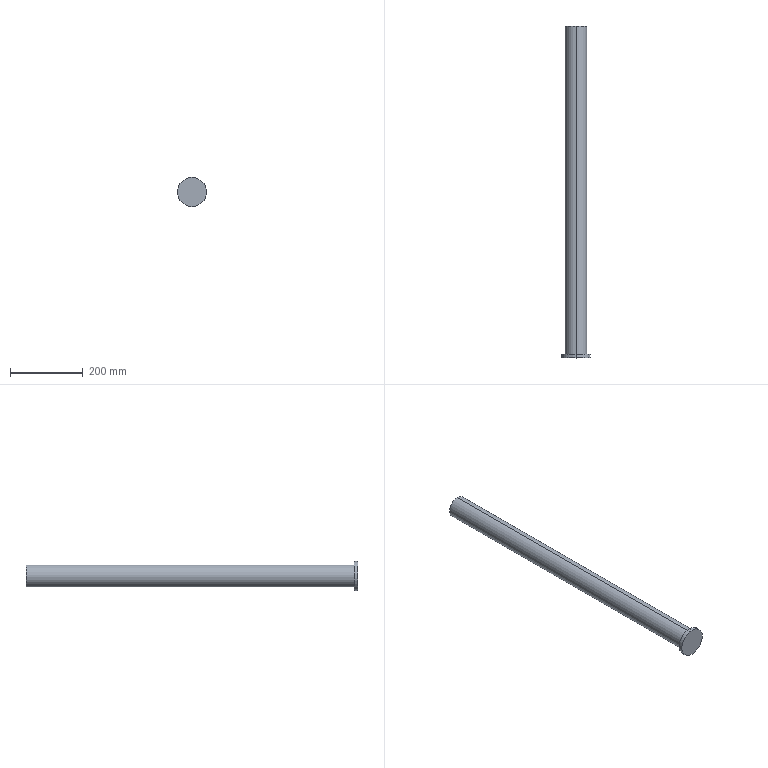Part | STEP file | Tie rod | 1 solid | 10 faces | box 80 x 910 x 80 mm | volume 827810 mm3 | cylinder 6 | plane 4 | commonest cylinder face diameters 50 x2 60 x2 80 x2
STEP:
#1=CARTESIAN_POINT('',(0.,910.,-25.));
#2=VERTEX_POINT('',#1);
#3=CARTESIAN_POINT('',(0.,910.,25.));
#4=VERTEX_POINT('',#3);
#5=CARTESIAN_POINT('',(0.,910.,0.));
#6=DIRECTION('',(0.,1.,0.));
#7=DIRECTION('',(0.,0.,1.));
#8=AXIS2_PLACEMENT_3D('',#5,#6,#7);
#9=CIRCLE('',#8,25.);
#10=EDGE_CURVE('',#2,#4,#9,.T.);
#11=ORIENTED_EDGE('',*,*,#10,.T.);
#12=CARTESIAN_POINT('',(0.,10.,25.));
#13=VERTEX_POINT('',#12);
#14=CARTESIAN_POINT('',(0.,910.,25.));
#15=DIRECTION('',(0.,-1.,0.));
#16=VECTOR('',#15,1000.);
#17=LINE('',#14,#16);
#18=EDGE_CURVE('',#4,#13,#17,.T.);
#19=ORIENTED_EDGE('',*,*,#18,.T.);
#20=CARTESIAN_POINT('',(0.,10.,-25.));
#21=VERTEX_POINT('',#20);
#22=CARTESIAN_POINT('',(0.,10.,0.));
#23=DIRECTION('',(0.,-1.,0.));
#24=DIRECTION('',(0.,0.,1.));
#25=AXIS2_PLACEMENT_3D('',#22,#23,#24);
#26=CIRCLE('',#25,25.);
#27=EDGE_CURVE('',#13,#21,#26,.T.);
#28=ORIENTED_EDGE('',*,*,#27,.T.);
#29=CARTESIAN_POINT('',(0.,910.,-25.));
#30=DIRECTION('',(0.,-1.,0.));
#31=VECTOR('',#30,1000.);
#32=LINE('',#29,#31);
#33=EDGE_CURVE('',#2,#21,#32,.T.);
#34=ORIENTED_EDGE('',*,*,#33,.F.);
#35=EDGE_LOOP('',(#11,#19,#28,#34));
#36=FACE_OUTER_BOUND('',#35,.T.);
#37=CARTESIAN_POINT('',(0.,910.,0.));
#38=DIRECTION('',(0.,-1.,0.));
#39=DIRECTION('',(0.,0.,-1.));
#40=AXIS2_PLACEMENT_3D('',#37,#38,#39);
#41=CYLINDRICAL_SURFACE('',#40,25.);
#42=ADVANCED_FACE('',(#36),#41,.F.);
#43=CARTESIAN_POINT('',(0.,910.,30.));
#44=VERTEX_POINT('',#43);
#45=CARTESIAN_POINT('',(0.,910.,-30.));
#46=VERTEX_POINT('',#45);
#47=CARTESIAN_POINT('',(0.,910.,0.));
#48=DIRECTION('',(0.,1.,0.));
#49=DIRECTION('',(0.,0.,1.));
#50=AXIS2_PLACEMENT_3D('',#47,#48,#49);
#51=CIRCLE('',#50,30.);
#52=EDGE_CURVE('',#44,#46,#51,.T.);
#53=ORIENTED_EDGE('',*,*,#52,.F.);
#54=CARTESIAN_POINT('',(0.,10.,30.));
#55=VERTEX_POINT('',#54);
#56=CARTESIAN_POINT('',(0.,910.,30.));
#57=DIRECTION('',(0.,-1.,0.));
#58=VECTOR('',#57,1000.);
#59=LINE('',#56,#58);
#60=EDGE_CURVE('',#44,#55,#59,.T.);
#61=ORIENTED_EDGE('',*,*,#60,.T.);
#62=CARTESIAN_POINT('',(0.,10.,-30.));
#63=VERTEX_POINT('',#62);
#64=CARTESIAN_POINT('',(0.,10.,0.));
#65=DIRECTION('',(0.,1.,0.));
#66=DIRECTION('',(0.,0.,1.));
#67=AXIS2_PLACEMENT_3D('',#64,#65,#66);
#68=CIRCLE('',#67,30.);
#69=EDGE_CURVE('',#55,#63,#68,.T.);
#70=ORIENTED_EDGE('',*,*,#69,.T.);
#71=CARTESIAN_POINT('',(0.,910.,-30.));
#72=DIRECTION('',(0.,-1.,0.));
#73=VECTOR('',#72,1000.);
#74=LINE('',#71,#73);
#75=EDGE_CURVE('',#46,#63,#74,.T.);
#76=ORIENTED_EDGE('',*,*,#75,.F.);
#77=EDGE_LOOP('',(#53,#61,#70,#76));
#78=FACE_OUTER_BOUND('',#77,.T.);
#79=CARTESIAN_POINT('',(0.,910.,0.));
#80=DIRECTION('',(0.,-1.,0.));
#81=DIRECTION('',(0.,0.,-1.));
#82=AXIS2_PLACEMENT_3D('',#79,#80,#81);
#83=CYLINDRICAL_SURFACE('',#82,30.);
#84=ADVANCED_FACE('',(#78),#83,.T.);
#85=CARTESIAN_POINT('',(0.,10.,40.));
#86=VERTEX_POINT('',#85);
#87=CARTESIAN_POINT('',(0.,10.,-40.));
#88=VERTEX_POINT('',#87);
#89=CARTESIAN_POINT('',(0.,10.,0.));
#90=DIRECTION('',(0.,1.,0.));
#91=DIRECTION('',(0.,0.,1.));
#92=AXIS2_PLACEMENT_3D('',#89,#90,#91);
#93=CIRCLE('',#92,40.);
#94=EDGE_CURVE('',#86,#88,#93,.T.);
#95=ORIENTED_EDGE('',*,*,#94,.F.);
#96=CARTESIAN_POINT('',(0.,0.,40.));
#97=VERTEX_POINT('',#96);
#98=CARTESIAN_POINT('',(0.,10.,40.));
#99=DIRECTION('',(0.,-1.,0.));
#100=VECTOR('',#99,1000.);
#101=LINE('',#98,#100);
#102=EDGE_CURVE('',#86,#97,#101,.T.);
#103=ORIENTED_EDGE('',*,*,#102,.T.);
#104=CARTESIAN_POINT('',(0.,0.,-40.));
#105=VERTEX_POINT('',#104);
#106=CARTESIAN_POINT('',(0.,0.,0.));
#107=DIRECTION('',(0.,1.,0.));
#108=DIRECTION('',(0.,0.,1.));
#109=AXIS2_PLACEMENT_3D('',#106,#107,#108);
#110=CIRCLE('',#109,40.);
#111=EDGE_CURVE('',#97,#105,#110,.T.);
#112=ORIENTED_EDGE('',*,*,#111,.T.);
#113=CARTESIAN_POINT('',(0.,10.,-40.));
#114=DIRECTION('',(0.,-1.,0.));
#115=VECTOR('',#114,1000.);
#116=LINE('',#113,#115);
#117=EDGE_CURVE('',#88,#105,#116,.T.);
#118=ORIENTED_EDGE('',*,*,#117,.F.);
#119=EDGE_LOOP('',(#95,#103,#112,#118));
#120=FACE_OUTER_BOUND('',#119,.T.);
#121=CARTESIAN_POINT('',(0.,10.,0.));
#122=DIRECTION('',(0.,-1.,0.));
#123=DIRECTION('',(0.,0.,-1.));
#124=AXIS2_PLACEMENT_3D('',#121,#122,#123);
#125=CYLINDRICAL_SURFACE('',#124,40.);
#126=ADVANCED_FACE('',(#120),#125,.T.);
#127=ORIENTED_EDGE('',*,*,#102,.F.);
#128=CARTESIAN_POINT('',(0.,10.,0.));
#129=DIRECTION('',(0.,1.,0.));
#130=DIRECTION('',(0.,0.,1.));
#131=AXIS2_PLACEMENT_3D('',#128,#129,#130);
#132=CIRCLE('',#131,40.);
#133=EDGE_CURVE('',#88,#86,#132,.T.);
#134=ORIENTED_EDGE('',*,*,#133,.F.);
#135=ORIENTED_EDGE('',*,*,#117,.T.);
#136=CARTESIAN_POINT('',(0.,0.,0.));
#137=DIRECTION('',(0.,1.,0.));
#138=DIRECTION('',(0.,0.,1.));
#139=AXIS2_PLACEMENT_3D('',#136,#137,#138);
#140=CIRCLE('',#139,40.);
#141=EDGE_CURVE('',#105,#97,#140,.T.);
#142=ORIENTED_EDGE('',*,*,#141,.T.);
#143=EDGE_LOOP('',(#127,#134,#135,#142));
#144=FACE_OUTER_BOUND('',#143,.T.);
#145=CARTESIAN_POINT('',(0.,10.,0.));
#146=DIRECTION('',(0.,-1.,0.));
#147=DIRECTION('',(0.,0.,-1.));
#148=AXIS2_PLACEMENT_3D('',#145,#146,#147);
#149=CYLINDRICAL_SURFACE('',#148,40.);
#150=ADVANCED_FACE('',(#144),#149,.T.);
#151=CARTESIAN_POINT('',(0.,10.,0.));
#152=DIRECTION('',(0.,1.,0.));
#153=DIRECTION('',(0.,0.,1.));
#154=AXIS2_PLACEMENT_3D('',#151,#152,#153);
#155=CIRCLE('',#154,30.);
#156=EDGE_CURVE('',#63,#55,#155,.T.);
#157=ORIENTED_EDGE('',*,*,#156,.F.);
#158=ORIENTED_EDGE('',*,*,#69,.F.);
#159=EDGE_LOOP('',(#157,#158));
#160=FACE_BOUND('',#159,.T.);
#161=ORIENTED_EDGE('',*,*,#133,.T.);
#162=ORIENTED_EDGE('',*,*,#94,.T.);
#163=EDGE_LOOP('',(#161,#162));
#164=FACE_OUTER_BOUND('',#163,.T.);
#165=CARTESIAN_POINT('',(0.,10.,0.));
#166=DIRECTION('',(0.,1.,0.));
#167=DIRECTION('',(0.,0.,1.));
#168=AXIS2_PLACEMENT_3D('',#165,#166,#167);
#169=PLANE('',#168);
#170=ADVANCED_FACE('',(#160,#164),#169,.T.);
#171=ORIENTED_EDGE('',*,*,#141,.F.);
#172=ORIENTED_EDGE('',*,*,#111,.F.);
#173=EDGE_LOOP('',(#171,#172));
#174=FACE_OUTER_BOUND('',#173,.T.);
#175=CARTESIAN_POINT('',(0.,0.,0.));
#176=DIRECTION('',(0.,1.,0.));
#177=DIRECTION('',(0.,0.,1.));
#178=AXIS2_PLACEMENT_3D('',#175,#176,#177);
#179=PLANE('',#178);
#180=ADVANCED_FACE('',(#174),#179,.F.);
#181=CARTESIAN_POINT('',(0.,910.,0.));
#182=DIRECTION('',(0.,1.,0.));
#183=DIRECTION('',(0.,0.,1.));
#184=AXIS2_PLACEMENT_3D('',#181,#182,#183);
#185=CIRCLE('',#184,30.);
#186=EDGE_CURVE('',#46,#44,#185,.T.);
#187=ORIENTED_EDGE('',*,*,#186,.T.);
#188=ORIENTED_EDGE('',*,*,#52,.T.);
#189=EDGE_LOOP('',(#187,#188));
#190=FACE_OUTER_BOUND('',#189,.T.);
#191=ORIENTED_EDGE('',*,*,#10,.F.);
#192=CARTESIAN_POINT('',(0.,910.,0.));
#193=DIRECTION('',(0.,1.,0.));
#194=DIRECTION('',(0.,0.,1.));
#195=AXIS2_PLACEMENT_3D('',#192,#193,#194);
#196=CIRCLE('',#195,25.);
#197=EDGE_CURVE('',#4,#2,#196,.T.);
#198=ORIENTED_EDGE('',*,*,#197,.F.);
#199=EDGE_LOOP('',(#191,#198));
#200=FACE_BOUND('',#199,.T.);
#201=CARTESIAN_POINT('',(0.,910.,0.));
#202=DIRECTION('',(0.,1.,0.));
#203=DIRECTION('',(0.,0.,1.));
#204=AXIS2_PLACEMENT_3D('',#201,#202,#203);
#205=PLANE('',#204);
#206=ADVANCED_FACE('',(#190,#200),#205,.T.);
#207=ORIENTED_EDGE('',*,*,#60,.F.);
#208=ORIENTED_EDGE('',*,*,#186,.F.);
#209=ORIENTED_EDGE('',*,*,#75,.T.);
#210=ORIENTED_EDGE('',*,*,#156,.T.);
#211=EDGE_LOOP('',(#207,#208,#209,#210));
#212=FACE_OUTER_BOUND('',#211,.T.);
#213=CARTESIAN_POINT('',(0.,910.,0.));
#214=DIRECTION('',(0.,-1.,0.));
#215=DIRECTION('',(0.,0.,-1.));
#216=AXIS2_PLACEMENT_3D('',#213,#214,#215);
#217=CYLINDRICAL_SURFACE('',#216,30.);
#218=ADVANCED_FACE('',(#212),#217,.T.);
#219=ORIENTED_EDGE('',*,*,#18,.F.);
#220=ORIENTED_EDGE('',*,*,#197,.T.);
#221=ORIENTED_EDGE('',*,*,#33,.T.);
#222=CARTESIAN_POINT('',(0.,10.,0.));
#223=DIRECTION('',(0.,-1.,0.));
#224=DIRECTION('',(0.,0.,1.));
#225=AXIS2_PLACEMENT_3D('',#222,#223,#224);
#226=CIRCLE('',#225,25.);
#227=EDGE_CURVE('',#21,#13,#226,.T.);
#228=ORIENTED_EDGE('',*,*,#227,.T.);
#229=EDGE_LOOP('',(#219,#220,#221,#228));
#230=FACE_OUTER_BOUND('',#229,.T.);
#231=CARTESIAN_POINT('',(0.,910.,0.));
#232=DIRECTION('',(0.,-1.,0.));
#233=DIRECTION('',(0.,0.,-1.));
#234=AXIS2_PLACEMENT_3D('',#231,#232,#233);
#235=CYLINDRICAL_SURFACE('',#234,25.);
#236=ADVANCED_FACE('',(#230),#235,.F.);
#237=ORIENTED_EDGE('',*,*,#227,.F.);
#238=ORIENTED_EDGE('',*,*,#27,.F.);
#239=EDGE_LOOP('',(#237,#238));
#240=FACE_OUTER_BOUND('',#239,.T.);
#241=CARTESIAN_POINT('',(0.,10.,0.));
#242=DIRECTION('',(0.,1.,0.));
#243=DIRECTION('',(0.,0.,1.));
#244=AXIS2_PLACEMENT_3D('',#241,#242,#243);
#245=PLANE('',#244);
#246=ADVANCED_FACE('',(#240),#245,.T.);
#247=CLOSED_SHELL('',(#42,#84,#126,#150,#170,#180,#206,#218,#236,#246));
#248=MANIFOLD_SOLID_BREP('',#247);
#249=CARTESIAN_POINT('',(0.,0.,0.));
#250=DIRECTION('',(0.,0.,1.));
#251=DIRECTION('',(1.,0.,0.));
#252=AXIS2_PLACEMENT_3D('',#249,#250,#251);
#253=(LENGTH_UNIT()NAMED_UNIT(*)SI_UNIT(.MILLI.,.METRE.));
#254=UNCERTAINTY_MEASURE_WITH_UNIT(LENGTH_MEASURE(0.00001),#253,'','');
#255=(NAMED_UNIT(*)PLANE_ANGLE_UNIT()SI_UNIT($,.RADIAN.));
#256=(NAMED_UNIT(*)SI_UNIT($,.STERADIAN.)SOLID_ANGLE_UNIT());
#257=(GEOMETRIC_REPRESENTATION_CONTEXT(3)GLOBAL_UNCERTAINTY_ASSIGNED_CONTEXT((#254))GLOBAL_UNIT_ASSIGNED_CONTEXT((#253,#255,#256))REPRESENTATION_CONTEXT('',''));
#258=ADVANCED_BREP_SHAPE_REPRESENTATION('',(#248,#252),#257);